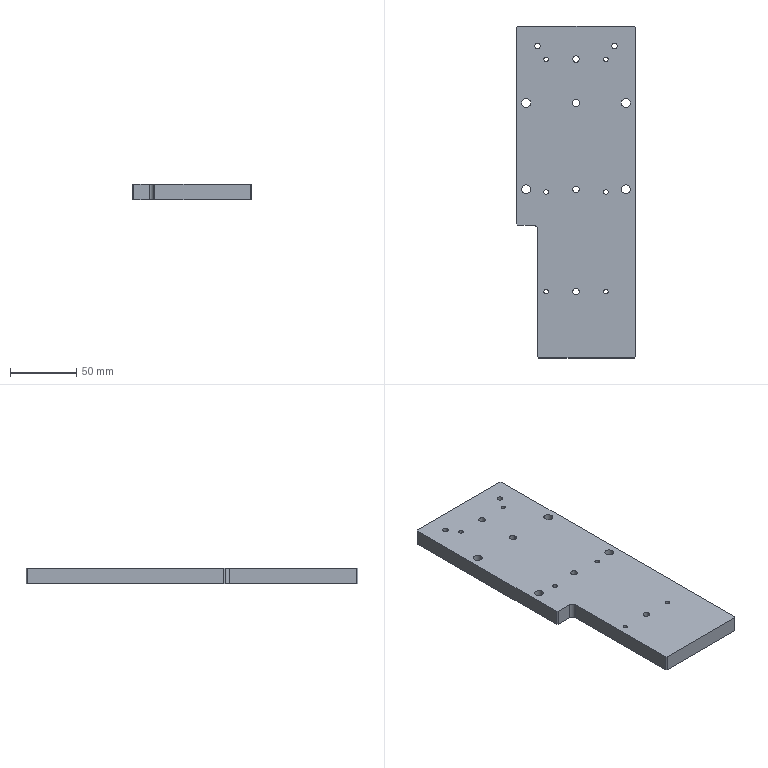Part | NX | 1 solid | 41 faces | box 90 x 250 x 12 mm | volume 245643 mm3 | cylinder 22 | plane 19 | commonest cylinder face diameters 3.3 x6 5 x5 6.6 x4 11 x4 4.2 x2 6 x1
STEP:
#1=CARTESIAN_POINT('',(-29.,97.,0.));
#2=VERTEX_POINT('',#1);
#3=CARTESIAN_POINT('',(-32.,100.,0.));
#4=VERTEX_POINT('',#3);
#5=CARTESIAN_POINT('',(-32.,97.,0.));
#6=DIRECTION('',(0.,0.,1.));
#7=DIRECTION('',(-1.,0.,0.));
#8=AXIS2_PLACEMENT_3D('',#5,#6,#7);
#9=CIRCLE('',#8,3.);
#10=EDGE_CURVE('',#2,#4,#9,.T.);
#11=ORIENTED_EDGE('',*,*,#10,.F.);
#12=CARTESIAN_POINT('',(-29.,97.,12.));
#13=VERTEX_POINT('',#12);
#14=CARTESIAN_POINT('',(-29.,97.,0.));
#15=DIRECTION('',(0.,0.,-1.));
#16=VECTOR('',#15,1000.);
#17=LINE('',#14,#16);
#18=EDGE_CURVE('',#13,#2,#17,.T.);
#19=ORIENTED_EDGE('',*,*,#18,.F.);
#20=CARTESIAN_POINT('',(-32.,100.,12.));
#21=VERTEX_POINT('',#20);
#22=CARTESIAN_POINT('',(-32.,97.,12.));
#23=DIRECTION('',(0.,0.,-1.));
#24=DIRECTION('',(-1.,0.,0.));
#25=AXIS2_PLACEMENT_3D('',#22,#23,#24);
#26=CIRCLE('',#25,3.);
#27=EDGE_CURVE('',#21,#13,#26,.T.);
#28=ORIENTED_EDGE('',*,*,#27,.F.);
#29=CARTESIAN_POINT('',(-32.,100.,12.));
#30=DIRECTION('',(0.,0.,1.));
#31=VECTOR('',#30,1000.);
#32=LINE('',#29,#31);
#33=EDGE_CURVE('',#4,#21,#32,.T.);
#34=ORIENTED_EDGE('',*,*,#33,.F.);
#35=EDGE_LOOP('',(#11,#19,#28,#34));
#36=FACE_BOUND('',#35,.T.);
#37=CARTESIAN_POINT('',(-32.,97.,0.));
#38=DIRECTION('',(0.,0.,-1.));
#39=DIRECTION('',(-1.,0.,0.));
#40=AXIS2_PLACEMENT_3D('',#37,#38,#39);
#41=CYLINDRICAL_SURFACE('',#40,3.);
#42=ADVANCED_FACE('',(#36),#41,.F.);
#43=CARTESIAN_POINT('',(45.,249.,12.));
#44=VERTEX_POINT('',#43);
#45=CARTESIAN_POINT('',(44.,250.,12.));
#46=VERTEX_POINT('',#45);
#47=CARTESIAN_POINT('',(44.,250.,12.));
#48=DIRECTION('',(-0.7071,0.7071,0.));
#49=VECTOR('',#48,1000.);
#50=LINE('',#47,#49);
#51=EDGE_CURVE('',#44,#46,#50,.T.);
#52=ORIENTED_EDGE('',*,*,#51,.F.);
#53=CARTESIAN_POINT('',(45.,249.,0.));
#54=VERTEX_POINT('',#53);
#55=CARTESIAN_POINT('',(45.,249.,12.));
#56=DIRECTION('',(0.,0.,1.));
#57=VECTOR('',#56,1000.);
#58=LINE('',#55,#57);
#59=EDGE_CURVE('',#54,#44,#58,.T.);
#60=ORIENTED_EDGE('',*,*,#59,.F.);
#61=CARTESIAN_POINT('',(44.,250.,0.));
#62=VERTEX_POINT('',#61);
#63=CARTESIAN_POINT('',(147.,147.,0.));
#64=DIRECTION('',(0.7071,-0.7071,0.));
#65=VECTOR('',#64,1000.);
#66=LINE('',#63,#65);
#67=EDGE_CURVE('',#62,#54,#66,.T.);
#68=ORIENTED_EDGE('',*,*,#67,.F.);
#69=CARTESIAN_POINT('',(44.,250.,12.));
#70=DIRECTION('',(0.,0.,-1.));
#71=VECTOR('',#70,1000.);
#72=LINE('',#69,#71);
#73=EDGE_CURVE('',#46,#62,#72,.T.);
#74=ORIENTED_EDGE('',*,*,#73,.F.);
#75=EDGE_LOOP('',(#52,#60,#68,#74));
#76=FACE_BOUND('',#75,.T.);
#77=CARTESIAN_POINT('',(44.,250.,12.));
#78=DIRECTION('',(-0.7071,-0.7071,0.));
#79=DIRECTION('',(0.,0.,-1.));
#80=AXIS2_PLACEMENT_3D('',#77,#78,#79);
#81=PLANE('',#80);
#82=ADVANCED_FACE('',(#76),#81,.F.);
#83=CARTESIAN_POINT('',(-44.,250.,12.));
#84=VERTEX_POINT('',#83);
#85=CARTESIAN_POINT('',(-45.,249.,12.));
#86=VERTEX_POINT('',#85);
#87=CARTESIAN_POINT('',(-45.,249.,12.));
#88=DIRECTION('',(-0.7071,-0.7071,0.));
#89=VECTOR('',#88,1000.);
#90=LINE('',#87,#89);
#91=EDGE_CURVE('',#84,#86,#90,.T.);
#92=ORIENTED_EDGE('',*,*,#91,.F.);
#93=CARTESIAN_POINT('',(-44.,250.,0.));
#94=VERTEX_POINT('',#93);
#95=CARTESIAN_POINT('',(-44.,250.,12.));
#96=DIRECTION('',(0.,0.,1.));
#97=VECTOR('',#96,1000.);
#98=LINE('',#95,#97);
#99=EDGE_CURVE('',#94,#84,#98,.T.);
#100=ORIENTED_EDGE('',*,*,#99,.F.);
#101=CARTESIAN_POINT('',(-45.,249.,0.));
#102=VERTEX_POINT('',#101);
#103=CARTESIAN_POINT('',(-147.,147.,0.));
#104=DIRECTION('',(0.7071,0.7071,0.));
#105=VECTOR('',#104,1000.);
#106=LINE('',#103,#105);
#107=EDGE_CURVE('',#102,#94,#106,.T.);
#108=ORIENTED_EDGE('',*,*,#107,.F.);
#109=CARTESIAN_POINT('',(-45.,249.,12.));
#110=DIRECTION('',(0.,0.,-1.));
#111=VECTOR('',#110,1000.);
#112=LINE('',#109,#111);
#113=EDGE_CURVE('',#86,#102,#112,.T.);
#114=ORIENTED_EDGE('',*,*,#113,.F.);
#115=EDGE_LOOP('',(#92,#100,#108,#114));
#116=FACE_BOUND('',#115,.T.);
#117=CARTESIAN_POINT('',(-45.,249.,12.));
#118=DIRECTION('',(0.7071,-0.7071,0.));
#119=DIRECTION('',(0.,0.,-1.));
#120=AXIS2_PLACEMENT_3D('',#117,#118,#119);
#121=PLANE('',#120);
#122=ADVANCED_FACE('',(#116),#121,.F.);
#123=CARTESIAN_POINT('',(44.,0.,12.));
#124=VERTEX_POINT('',#123);
#125=CARTESIAN_POINT('',(45.,1.,12.));
#126=VERTEX_POINT('',#125);
#127=CARTESIAN_POINT('',(45.,1.,12.));
#128=DIRECTION('',(0.7071,0.7071,0.));
#129=VECTOR('',#128,1000.);
#130=LINE('',#127,#129);
#131=EDGE_CURVE('',#124,#126,#130,.T.);
#132=ORIENTED_EDGE('',*,*,#131,.F.);
#133=CARTESIAN_POINT('',(44.,0.,0.));
#134=VERTEX_POINT('',#133);
#135=CARTESIAN_POINT('',(44.,0.,12.));
#136=DIRECTION('',(0.,0.,1.));
#137=VECTOR('',#136,1000.);
#138=LINE('',#135,#137);
#139=EDGE_CURVE('',#134,#124,#138,.T.);
#140=ORIENTED_EDGE('',*,*,#139,.F.);
#141=CARTESIAN_POINT('',(45.,1.,0.));
#142=VERTEX_POINT('',#141);
#143=CARTESIAN_POINT('',(22.,-22.,0.));
#144=DIRECTION('',(-0.7071,-0.7071,0.));
#145=VECTOR('',#144,1000.);
#146=LINE('',#143,#145);
#147=EDGE_CURVE('',#142,#134,#146,.T.);
#148=ORIENTED_EDGE('',*,*,#147,.F.);
#149=CARTESIAN_POINT('',(45.,1.,12.));
#150=DIRECTION('',(0.,0.,-1.));
#151=VECTOR('',#150,1000.);
#152=LINE('',#149,#151);
#153=EDGE_CURVE('',#126,#142,#152,.T.);
#154=ORIENTED_EDGE('',*,*,#153,.F.);
#155=EDGE_LOOP('',(#132,#140,#148,#154));
#156=FACE_BOUND('',#155,.T.);
#157=CARTESIAN_POINT('',(45.,1.,12.));
#158=DIRECTION('',(-0.7071,0.7071,0.));
#159=DIRECTION('',(0.,0.,-1.));
#160=AXIS2_PLACEMENT_3D('',#157,#158,#159);
#161=PLANE('',#160);
#162=ADVANCED_FACE('',(#156),#161,.F.);
#163=CARTESIAN_POINT('',(-44.,100.,0.));
#164=VERTEX_POINT('',#163);
#165=CARTESIAN_POINT('',(-45.,101.,0.));
#166=VERTEX_POINT('',#165);
#167=CARTESIAN_POINT('',(28.,28.,0.));
#168=DIRECTION('',(-0.7071,0.7071,0.));
#169=VECTOR('',#168,1000.);
#170=LINE('',#167,#169);
#171=EDGE_CURVE('',#164,#166,#170,.T.);
#172=ORIENTED_EDGE('',*,*,#171,.F.);
#173=CARTESIAN_POINT('',(-44.,100.,12.));
#174=VERTEX_POINT('',#173);
#175=CARTESIAN_POINT('',(-44.,100.,0.));
#176=DIRECTION('',(0.,0.,-1.));
#177=VECTOR('',#176,1000.);
#178=LINE('',#175,#177);
#179=EDGE_CURVE('',#174,#164,#178,.T.);
#180=ORIENTED_EDGE('',*,*,#179,.F.);
#181=CARTESIAN_POINT('',(-45.,101.,12.));
#182=VERTEX_POINT('',#181);
#183=CARTESIAN_POINT('',(-45.,101.,12.));
#184=DIRECTION('',(0.7071,-0.7071,0.));
#185=VECTOR('',#184,1000.);
#186=LINE('',#183,#185);
#187=EDGE_CURVE('',#182,#174,#186,.T.);
#188=ORIENTED_EDGE('',*,*,#187,.F.);
#189=CARTESIAN_POINT('',(-45.,101.,12.));
#190=DIRECTION('',(0.,0.,1.));
#191=VECTOR('',#190,1000.);
#192=LINE('',#189,#191);
#193=EDGE_CURVE('',#166,#182,#192,.T.);
#194=ORIENTED_EDGE('',*,*,#193,.F.);
#195=EDGE_LOOP('',(#172,#180,#188,#194));
#196=FACE_BOUND('',#195,.T.);
#197=CARTESIAN_POINT('',(-45.,101.,12.));
#198=DIRECTION('',(0.7071,0.7071,0.));
#199=DIRECTION('',(0.,0.,1.));
#200=AXIS2_PLACEMENT_3D('',#197,#198,#199);
#201=PLANE('',#200);
#202=ADVANCED_FACE('',(#196),#201,.F.);
#203=CARTESIAN_POINT('',(-28.,0.,0.));
#204=VERTEX_POINT('',#203);
#205=CARTESIAN_POINT('',(-29.,1.,0.));
#206=VERTEX_POINT('',#205);
#207=CARTESIAN_POINT('',(-14.,-14.,0.));
#208=DIRECTION('',(-0.7071,0.7071,0.));
#209=VECTOR('',#208,1000.);
#210=LINE('',#207,#209);
#211=EDGE_CURVE('',#204,#206,#210,.T.);
#212=ORIENTED_EDGE('',*,*,#211,.F.);
#213=CARTESIAN_POINT('',(-28.,0.,12.));
#214=VERTEX_POINT('',#213);
#215=CARTESIAN_POINT('',(-28.,0.,12.));
#216=DIRECTION('',(0.,0.,-1.));
#217=VECTOR('',#216,1000.);
#218=LINE('',#215,#217);
#219=EDGE_CURVE('',#214,#204,#218,.T.);
#220=ORIENTED_EDGE('',*,*,#219,.F.);
#221=CARTESIAN_POINT('',(-29.,1.,12.));
#222=VERTEX_POINT('',#221);
#223=CARTESIAN_POINT('',(-29.,1.,12.));
#224=DIRECTION('',(0.7071,-0.7071,0.));
#225=VECTOR('',#224,1000.);
#226=LINE('',#223,#225);
#227=EDGE_CURVE('',#222,#214,#226,.T.);
#228=ORIENTED_EDGE('',*,*,#227,.F.);
#229=CARTESIAN_POINT('',(-29.,1.,0.));
#230=DIRECTION('',(0.,0.,1.));
#231=VECTOR('',#230,1000.);
#232=LINE('',#229,#231);
#233=EDGE_CURVE('',#206,#222,#232,.T.);
#234=ORIENTED_EDGE('',*,*,#233,.F.);
#235=EDGE_LOOP('',(#212,#220,#228,#234));
#236=FACE_BOUND('',#235,.T.);
#237=CARTESIAN_POINT('',(-29.,1.,0.));
#238=DIRECTION('',(0.7071,0.7071,0.));
#239=DIRECTION('',(0.,0.,1.));
#240=AXIS2_PLACEMENT_3D('',#237,#238,#239);
#241=PLANE('',#240);
#242=ADVANCED_FACE('',(#236),#241,.F.);
#243=CARTESIAN_POINT('',(-29.,100.,12.));
#244=DIRECTION('',(0.,1.,0.));
#245=VECTOR('',#244,1000.);
#246=LINE('',#243,#245);
#247=EDGE_CURVE('',#222,#13,#246,.T.);
#248=ORIENTED_EDGE('',*,*,#247,.T.);
#249=ORIENTED_EDGE('',*,*,#18,.T.);
#250=CARTESIAN_POINT('',(-29.,100.,0.));
#251=DIRECTION('',(0.,1.,0.));
#252=VECTOR('',#251,1000.);
#253=LINE('',#250,#252);
#254=EDGE_CURVE('',#206,#2,#253,.T.);
#255=ORIENTED_EDGE('',*,*,#254,.F.);
#256=ORIENTED_EDGE('',*,*,#233,.T.);
#257=EDGE_LOOP('',(#248,#249,#255,#256));
#258=FACE_BOUND('',#257,.T.);
#259=CARTESIAN_POINT('',(-29.,100.,0.));
#260=DIRECTION('',(1.,0.,0.));
#261=DIRECTION('',(0.,1.,0.));
#262=AXIS2_PLACEMENT_3D('',#259,#260,#261);
#263=PLANE('',#262);
#264=ADVANCED_FACE('',(#258),#263,.F.);
#265=CARTESIAN_POINT('',(-45.,100.,0.));
#266=DIRECTION('',(-1.,0.,0.));
#267=VECTOR('',#266,1000.);
#268=LINE('',#265,#267);
#269=EDGE_CURVE('',#4,#164,#268,.T.);
#270=ORIENTED_EDGE('',*,*,#269,.F.);
#271=ORIENTED_EDGE('',*,*,#33,.T.);
#272=CARTESIAN_POINT('',(-45.,100.,12.));
#273=DIRECTION('',(-1.,0.,0.));
#274=VECTOR('',#273,1000.);
#275=LINE('',#272,#274);
#276=EDGE_CURVE('',#21,#174,#275,.T.);
#277=ORIENTED_EDGE('',*,*,#276,.T.);
#278=ORIENTED_EDGE('',*,*,#179,.T.);
#279=EDGE_LOOP('',(#270,#271,#277,#278));
#280=FACE_BOUND('',#279,.T.);
#281=CARTESIAN_POINT('',(-45.,100.,0.));
#282=DIRECTION('',(0.,1.,0.));
#283=DIRECTION('',(0.,0.,1.));
#284=AXIS2_PLACEMENT_3D('',#281,#282,#283);
#285=PLANE('',#284);
#286=ADVANCED_FACE('',(#280),#285,.F.);
#287=CARTESIAN_POINT('',(-2.5,192.5,0.));
#288=VERTEX_POINT('',#287);
#289=CARTESIAN_POINT('',(-2.5,192.5,12.));
#290=VERTEX_POINT('',#289);
#291=CARTESIAN_POINT('',(-2.5,192.5,0.));
#292=DIRECTION('',(0.,0.,1.));
#293=VECTOR('',#292,1000.);
#294=LINE('',#291,#293);
#295=EDGE_CURVE('',#288,#290,#294,.T.);
#296=ORIENTED_EDGE('',*,*,#295,.T.);
#297=CARTESIAN_POINT('',(-2.5,191.5,12.));
#298=VERTEX_POINT('',#297);
#299=CARTESIAN_POINT('',(-2.5,191.5,12.));
#300=DIRECTION('',(0.,1.,0.));
#301=VECTOR('',#300,1000.);
#302=LINE('',#299,#301);
#303=EDGE_CURVE('',#298,#290,#302,.T.);
#304=ORIENTED_EDGE('',*,*,#303,.F.);
#305=CARTESIAN_POINT('',(-2.5,191.5,0.));
#306=VERTEX_POINT('',#305);
#307=CARTESIAN_POINT('',(-2.5,191.5,0.));
#308=DIRECTION('',(0.,0.,-1.));
#309=VECTOR('',#308,1000.);
#310=LINE('',#307,#309);
#311=EDGE_CURVE('',#298,#306,#310,.T.);
#312=ORIENTED_EDGE('',*,*,#311,.T.);
#313=CARTESIAN_POINT('',(-2.5,191.5,0.));
#314=DIRECTION('',(0.,1.,0.));
#315=VECTOR('',#314,1000.);
#316=LINE('',#313,#315);
#317=EDGE_CURVE('',#306,#288,#316,.T.);
#318=ORIENTED_EDGE('',*,*,#317,.T.);
#319=EDGE_LOOP('',(#296,#304,#312,#318));
#320=FACE_BOUND('',#319,.T.);
#321=CARTESIAN_POINT('',(-2.5,191.5,0.));
#322=DIRECTION('',(-1.,0.,0.));
#323=DIRECTION('',(0.,0.,1.));
#324=AXIS2_PLACEMENT_3D('',#321,#322,#323);
#325=PLANE('',#324);
#326=ADVANCED_FACE('',(#320),#325,.F.);
#327=CARTESIAN_POINT('',(2.5,192.5,0.));
#328=VERTEX_POINT('',#327);
#329=CARTESIAN_POINT('',(2.5,192.5,12.));
#330=VERTEX_POINT('',#329);
#331=CARTESIAN_POINT('',(2.5,192.5,12.));
#332=DIRECTION('',(0.,0.,1.));
#333=VECTOR('',#332,1000.);
#334=LINE('',#331,#333);
#335=EDGE_CURVE('',#328,#330,#334,.T.);
#336=ORIENTED_EDGE('',*,*,#335,.F.);
#337=CARTESIAN_POINT('',(2.5,191.5,0.));
#338=VERTEX_POINT('',#337);
#339=CARTESIAN_POINT('',(2.5,191.5,0.));
#340=DIRECTION('',(0.,1.,0.));
#341=VECTOR('',#340,1000.);
#342=LINE('',#339,#341);
#343=EDGE_CURVE('',#338,#328,#342,.T.);
#344=ORIENTED_EDGE('',*,*,#343,.F.);
#345=CARTESIAN_POINT('',(2.5,191.5,12.));
#346=VERTEX_POINT('',#345);
#347=CARTESIAN_POINT('',(2.5,191.5,12.));
#348=DIRECTION('',(0.,0.,1.));
#349=VECTOR('',#348,1000.);
#350=LINE('',#347,#349);
#351=EDGE_CURVE('',#338,#346,#350,.T.);
#352=ORIENTED_EDGE('',*,*,#351,.T.);
#353=CARTESIAN_POINT('',(2.5,191.5,12.));
#354=DIRECTION('',(0.,1.,0.));
#355=VECTOR('',#354,1000.);
#356=LINE('',#353,#355);
#357=EDGE_CURVE('',#346,#330,#356,.T.);
#358=ORIENTED_EDGE('',*,*,#357,.T.);
#359=EDGE_LOOP('',(#336,#344,#352,#358));
#360=FACE_BOUND('',#359,.T.);
#361=CARTESIAN_POINT('',(2.5,191.5,12.));
#362=DIRECTION('',(-1.,0.,0.));
#363=DIRECTION('',(0.,0.,1.));
#364=AXIS2_PLACEMENT_3D('',#361,#362,#363);
#365=PLANE('',#364);
#366=ADVANCED_FACE('',(#360),#365,.T.);
#367=CARTESIAN_POINT('',(0.,191.5,12.));
#368=DIRECTION('',(0.,0.,-1.));
#369=DIRECTION('',(-1.,0.,0.));
#370=AXIS2_PLACEMENT_3D('',#367,#368,#369);
#371=CIRCLE('',#370,2.5);
#372=EDGE_CURVE('',#346,#298,#371,.T.);
#373=ORIENTED_EDGE('',*,*,#372,.F.);
#374=ORIENTED_EDGE('',*,*,#351,.F.);
#375=CARTESIAN_POINT('',(0.,191.5,0.));
#376=DIRECTION('',(0.,0.,-1.));
#377=DIRECTION('',(-1.,0.,0.));
#378=AXIS2_PLACEMENT_3D('',#375,#376,#377);
#379=CIRCLE('',#378,2.5);
#380=EDGE_CURVE('',#338,#306,#379,.T.);
#381=ORIENTED_EDGE('',*,*,#380,.T.);
#382=ORIENTED_EDGE('',*,*,#311,.F.);
#383=EDGE_LOOP('',(#373,#374,#381,#382));
#384=FACE_BOUND('',#383,.T.);
#385=CARTESIAN_POINT('',(0.,191.5,0.));
#386=DIRECTION('',(0.,0.,-1.));
#387=DIRECTION('',(-1.,0.,0.));
#388=AXIS2_PLACEMENT_3D('',#385,#386,#387);
#389=CYLINDRICAL_SURFACE('',#388,2.5);
#390=ADVANCED_FACE('',(#384),#389,.F.);
#391=CARTESIAN_POINT('',(0.,192.5,0.));
#392=DIRECTION('',(0.,0.,-1.));
#393=DIRECTION('',(-1.,0.,0.));
#394=AXIS2_PLACEMENT_3D('',#391,#392,#393);
#395=CIRCLE('',#394,2.5);
#396=EDGE_CURVE('',#288,#328,#395,.T.);
#397=ORIENTED_EDGE('',*,*,#396,.T.);
#398=ORIENTED_EDGE('',*,*,#335,.T.);
#399=CARTESIAN_POINT('',(0.,192.5,12.));
#400=DIRECTION('',(0.,0.,-1.));
#401=DIRECTION('',(-1.,0.,0.));
#402=AXIS2_PLACEMENT_3D('',#399,#400,#401);
#403=CIRCLE('',#402,2.5);
#404=EDGE_CURVE('',#290,#330,#403,.T.);
#405=ORIENTED_EDGE('',*,*,#404,.F.);
#406=ORIENTED_EDGE('',*,*,#295,.F.);
#407=EDGE_LOOP('',(#397,#398,#405,#406));
#408=FACE_BOUND('',#407,.T.);
#409=CARTESIAN_POINT('',(0.,192.5,0.));
#410=DIRECTION('',(0.,0.,-1.));
#411=DIRECTION('',(-1.,0.,0.));
#412=AXIS2_PLACEMENT_3D('',#409,#410,#411);
#413=CYLINDRICAL_SURFACE('',#412,2.5);
#414=ADVANCED_FACE('',(#408),#413,.F.);
#415=CARTESIAN_POINT('',(32.,127.,6.4));
#416=VERTEX_POINT('',#415);
#417=CARTESIAN_POINT('',(37.5,127.,6.4));
#418=DIRECTION('',(0.,0.,-1.));
#419=DIRECTION('',(-1.,0.,0.));
#420=AXIS2_PLACEMENT_3D('',#417,#418,#419);
#421=CIRCLE('',#420,5.5);
#422=EDGE_CURVE('',#416,#416,#421,.T.);
#423=ORIENTED_EDGE('',*,*,#422,.T.);
#424=EDGE_LOOP('',(#423));
#425=FACE_BOUND('',#424,.T.);
#426=CARTESIAN_POINT('',(34.2,127.,6.4));
#427=VERTEX_POINT('',#426);
#428=CARTESIAN_POINT('',(37.5,127.,6.4));
#429=DIRECTION('',(0.,0.,-1.));
#430=DIRECTION('',(-1.,0.,0.));
#431=AXIS2_PLACEMENT_3D('',#428,#429,#430);
#432=CIRCLE('',#431,3.3);
#433=EDGE_CURVE('',#427,#427,#432,.T.);
#434=ORIENTED_EDGE('',*,*,#433,.F.);
#435=EDGE_LOOP('',(#434));
#436=FACE_BOUND('',#435,.T.);
#437=CARTESIAN_POINT('',(40.8,127.,6.4));
#438=DIRECTION('',(0.,0.,1.));
#439=DIRECTION('',(1.,0.,0.));
#440=AXIS2_PLACEMENT_3D('',#437,#438,#439);
#441=PLANE('',#440);
#442=ADVANCED_FACE('',(#425,#436),#441,.F.);
#443=CARTESIAN_POINT('',(-32.,192.,6.4));
#444=VERTEX_POINT('',#443);
#445=CARTESIAN_POINT('',(-37.5,192.,6.4));
#446=DIRECTION('',(0.,0.,-1.));
#447=DIRECTION('',(1.,0.,0.));
#448=AXIS2_PLACEMENT_3D('',#445,#446,#447);
#449=CIRCLE('',#448,5.5);
#450=EDGE_CURVE('',#444,#444,#449,.T.);
#451=ORIENTED_EDGE('',*,*,#450,.T.);
#452=EDGE_LOOP('',(#451));
#453=FACE_BOUND('',#452,.T.);
#454=CARTESIAN_POINT('',(-34.2,192.,6.4));
#455=VERTEX_POINT('',#454);
#456=CARTESIAN_POINT('',(-37.5,192.,6.4));
#457=DIRECTION('',(0.,0.,-1.));
#458=DIRECTION('',(1.,0.,0.));
#459=AXIS2_PLACEMENT_3D('',#456,#457,#458);
#460=CIRCLE('',#459,3.3);
#461=EDGE_CURVE('',#455,#455,#460,.T.);
#462=ORIENTED_EDGE('',*,*,#461,.F.);
#463=EDGE_LOOP('',(#462));
#464=FACE_BOUND('',#463,.T.);
#465=CARTESIAN_POINT('',(40.8,127.,6.4));
#466=DIRECTION('',(0.,0.,1.));
#467=DIRECTION('',(1.,0.,0.));
#468=AXIS2_PLACEMENT_3D('',#465,#466,#467);
#469=PLANE('',#468);
#470=ADVANCED_FACE('',(#453,#464),#469,.F.);
#471=CARTESIAN_POINT('',(43.,192.,6.4));
#472=VERTEX_POINT('',#471);
#473=CARTESIAN_POINT('',(37.5,192.,6.4));
#474=DIRECTION('',(0.,0.,-1.));
#475=DIRECTION('',(1.,0.,0.));
#476=AXIS2_PLACEMENT_3D('',#473,#474,#475);
#477=CIRCLE('',#476,5.5);
#478=EDGE_CURVE('',#472,#472,#477,.T.);
#479=ORIENTED_EDGE('',*,*,#478,.T.);
#480=EDGE_LOOP('',(#479));
#481=FACE_BOUND('',#480,.T.);
#482=CARTESIAN_POINT('',(40.8,192.,6.4));
#483=VERTEX_POINT('',#482);
#484=CARTESIAN_POINT('',(37.5,192.,6.4));
#485=DIRECTION('',(0.,0.,-1.));
#486=DIRECTION('',(1.,0.,0.));
#487=AXIS2_PLACEMENT_3D('',#484,#485,#486);
#488=CIRCLE('',#487,3.3);
#489=EDGE_CURVE('',#483,#483,#488,.T.);
#490=ORIENTED_EDGE('',*,*,#489,.F.);
#491=EDGE_LOOP('',(#490));
#492=FACE_BOUND('',#491,.T.);
#493=CARTESIAN_POINT('',(40.8,127.,6.4));
#494=DIRECTION('',(0.,0.,1.));
#495=DIRECTION('',(1.,0.,0.));
#496=AXIS2_PLACEMENT_3D('',#493,#494,#495);
#497=PLANE('',#496);
#498=ADVANCED_FACE('',(#481,#492),#497,.F.);
#499=CARTESIAN_POINT('',(-32.,127.,6.4));
#500=VERTEX_POINT('',#499);
#501=CARTESIAN_POINT('',(-37.5,127.,6.4));
#502=DIRECTION('',(0.,0.,-1.));
#503=DIRECTION('',(1.,0.,0.));
#504=AXIS2_PLACEMENT_3D('',#501,#502,#503);
#505=CIRCLE('',#504,5.5);
#506=EDGE_CURVE('',#500,#500,#505,.T.);
#507=ORIENTED_EDGE('',*,*,#506,.T.);
#508=EDGE_LOOP('',(#507));
#509=FACE_BOUND('',#508,.T.);
#510=CARTESIAN_POINT('',(-34.2,127.,6.4));
#511=VERTEX_POINT('',#510);
#512=CARTESIAN_POINT('',(-37.5,127.,6.4));
#513=DIRECTION('',(0.,0.,-1.));
#514=DIRECTION('',(1.,0.,0.));
#515=AXIS2_PLACEMENT_3D('',#512,#513,#514);
#516=CIRCLE('',#515,3.3);
#517=EDGE_CURVE('',#511,#511,#516,.T.);
#518=ORIENTED_EDGE('',*,*,#517,.F.);
#519=EDGE_LOOP('',(#518));
#520=FACE_BOUND('',#519,.T.);
#521=CARTESIAN_POINT('',(40.8,127.,6.4));
#522=DIRECTION('',(0.,0.,1.));
#523=DIRECTION('',(1.,0.,0.));
#524=AXIS2_PLACEMENT_3D('',#521,#522,#523);
#525=PLANE('',#524);
#526=ADVANCED_FACE('',(#509,#520),#525,.F.);
#527=ORIENTED_EDGE('',*,*,#247,.F.);
#528=ORIENTED_EDGE('',*,*,#227,.T.);
#529=CARTESIAN_POINT('',(-45.,0.,12.));
#530=DIRECTION('',(1.,0.,0.));
#531=VECTOR('',#530,1000.);
#532=LINE('',#529,#531);
#533=EDGE_CURVE('',#214,#124,#532,.T.);
#534=ORIENTED_EDGE('',*,*,#533,.T.);
#535=ORIENTED_EDGE('',*,*,#131,.T.);
#536=CARTESIAN_POINT('',(45.,0.,12.));
#537=DIRECTION('',(0.,1.,0.));
#538=VECTOR('',#537,1000.);
#539=LINE('',#536,#538);
#540=EDGE_CURVE('',#126,#44,#539,.T.);
#541=ORIENTED_EDGE('',*,*,#540,.T.);
#542=ORIENTED_EDGE('',*,*,#51,.T.);
#543=CARTESIAN_POINT('',(-45.,250.,12.));
#544=DIRECTION('',(-1.,0.,0.));
#545=VECTOR('',#544,1000.);
#546=LINE('',#543,#545);
#547=EDGE_CURVE('',#46,#84,#546,.T.);
#548=ORIENTED_EDGE('',*,*,#547,.T.);
#549=ORIENTED_EDGE('',*,*,#91,.T.);
#550=CARTESIAN_POINT('',(-45.,0.,12.));
#551=DIRECTION('',(0.,-1.,0.));
#552=VECTOR('',#551,1000.);
#553=LINE('',#550,#552);
#554=EDGE_CURVE('',#86,#182,#553,.T.);
#555=ORIENTED_EDGE('',*,*,#554,.T.);
#556=ORIENTED_EDGE('',*,*,#187,.T.);
#557=ORIENTED_EDGE('',*,*,#276,.F.);
#558=ORIENTED_EDGE('',*,*,#27,.T.);
#559=EDGE_LOOP('',(#527,#528,#534,#535,#541,#542,#548,#549,#555,#556,#557,#558));
#560=FACE_BOUND('',#559,.T.);
#561=CARTESIAN_POINT('',(-24.15,125.,12.));
#562=VERTEX_POINT('',#561);
#563=CARTESIAN_POINT('',(-22.5,125.,12.));
#564=DIRECTION('',(0.,0.,-1.));
#565=DIRECTION('',(-1.,0.,0.));
#566=AXIS2_PLACEMENT_3D('',#563,#564,#565);
#567=CIRCLE('',#566,1.65);
#568=EDGE_CURVE('',#562,#562,#567,.T.);
#569=ORIENTED_EDGE('',*,*,#568,.T.);
#570=EDGE_LOOP('',(#569));
#571=FACE_BOUND('',#570,.T.);
#572=CARTESIAN_POINT('',(-24.15,50.,12.));
#573=VERTEX_POINT('',#572);
#574=CARTESIAN_POINT('',(-22.5,50.,12.));
#575=DIRECTION('',(0.,0.,-1.));
#576=DIRECTION('',(-1.,0.,0.));
#577=AXIS2_PLACEMENT_3D('',#574,#575,#576);
#578=CIRCLE('',#577,1.65);
#579=EDGE_CURVE('',#573,#573,#578,.T.);
#580=ORIENTED_EDGE('',*,*,#579,.T.);
#581=EDGE_LOOP('',(#580));
#582=FACE_BOUND('',#581,.T.);
#583=CARTESIAN_POINT('',(20.85,125.,12.));
#584=VERTEX_POINT('',#583);
#585=CARTESIAN_POINT('',(22.5,125.,12.));
#586=DIRECTION('',(0.,0.,-1.));
#587=DIRECTION('',(-1.,0.,0.));
#588=AXIS2_PLACEMENT_3D('',#585,#586,#587);
#589=CIRCLE('',#588,1.65);
#590=EDGE_CURVE('',#584,#584,#589,.T.);
#591=ORIENTED_EDGE('',*,*,#590,.T.);
#592=EDGE_LOOP('',(#591));
#593=FACE_BOUND('',#592,.T.);
#594=CARTESIAN_POINT('',(20.85,50.,12.));
#595=VERTEX_POINT('',#594);
#596=CARTESIAN_POINT('',(22.5,50.,12.));
#597=DIRECTION('',(0.,0.,-1.));
#598=DIRECTION('',(-1.,0.,0.));
#599=AXIS2_PLACEMENT_3D('',#596,#597,#598);
#600=CIRCLE('',#599,1.65);
#601=EDGE_CURVE('',#595,#595,#600,.T.);
#602=ORIENTED_EDGE('',*,*,#601,.T.);
#603=EDGE_LOOP('',(#602));
#604=FACE_BOUND('',#603,.T.);
#605=CARTESIAN_POINT('',(20.85,225.,12.));
#606=VERTEX_POINT('',#605);
#607=CARTESIAN_POINT('',(22.5,225.,12.));
#608=DIRECTION('',(0.,0.,-1.));
#609=DIRECTION('',(-1.,0.,0.));
#610=AXIS2_PLACEMENT_3D('',#607,#608,#609);
#611=CIRCLE('',#610,1.65);
#612=EDGE_CURVE('',#606,#606,#611,.T.);
#613=ORIENTED_EDGE('',*,*,#612,.T.);
#614=EDGE_LOOP('',(#613));
#615=FACE_BOUND('',#614,.T.);
#616=CARTESIAN_POINT('',(-24.15,225.,12.));
#617=VERTEX_POINT('',#616);
#618=CARTESIAN_POINT('',(-22.5,225.,12.));
#619=DIRECTION('',(0.,0.,-1.));
#620=DIRECTION('',(-1.,0.,0.));
#621=AXIS2_PLACEMENT_3D('',#618,#619,#620);
#622=CIRCLE('',#621,1.65);
#623=EDGE_CURVE('',#617,#617,#622,.T.);
#624=ORIENTED_EDGE('',*,*,#623,.T.);
#625=EDGE_LOOP('',(#624));
#626=FACE_BOUND('',#625,.T.);
#627=CARTESIAN_POINT('',(31.1,235.,12.));
#628=VERTEX_POINT('',#627);
#629=CARTESIAN_POINT('',(29.,235.,12.));
#630=DIRECTION('',(0.,0.,1.));
#631=DIRECTION('',(1.,0.,0.));
#632=AXIS2_PLACEMENT_3D('',#629,#630,#631);
#633=CIRCLE('',#632,2.1);
#634=EDGE_CURVE('',#628,#628,#633,.T.);
#635=ORIENTED_EDGE('',*,*,#634,.F.);
#636=EDGE_LOOP('',(#635));
#637=FACE_BOUND('',#636,.T.);
#638=CARTESIAN_POINT('',(-26.9,235.,12.));
#639=VERTEX_POINT('',#638);
#640=CARTESIAN_POINT('',(-29.,235.,12.));
#641=DIRECTION('',(0.,0.,1.));
#642=DIRECTION('',(1.,0.,0.));
#643=AXIS2_PLACEMENT_3D('',#640,#641,#642);
#644=CIRCLE('',#643,2.1);
#645=EDGE_CURVE('',#639,#639,#644,.T.);
#646=ORIENTED_EDGE('',*,*,#645,.F.);
#647=EDGE_LOOP('',(#646));
#648=FACE_BOUND('',#647,.T.);
#649=CARTESIAN_POINT('',(-40.8,127.,12.));
#650=VERTEX_POINT('',#649);
#651=CARTESIAN_POINT('',(-37.5,127.,12.));
#652=DIRECTION('',(0.,0.,-1.));
#653=DIRECTION('',(-1.,0.,0.));
#654=AXIS2_PLACEMENT_3D('',#651,#652,#653);
#655=CIRCLE('',#654,3.3);
#656=EDGE_CURVE('',#650,#650,#655,.T.);
#657=ORIENTED_EDGE('',*,*,#656,.T.);
#658=EDGE_LOOP('',(#657));
#659=FACE_BOUND('',#658,.T.);
#660=CARTESIAN_POINT('',(34.2,192.,12.));
#661=VERTEX_POINT('',#660);
#662=CARTESIAN_POINT('',(37.5,192.,12.));
#663=DIRECTION('',(0.,0.,-1.));
#664=DIRECTION('',(-1.,0.,0.));
#665=AXIS2_PLACEMENT_3D('',#662,#663,#664);
#666=CIRCLE('',#665,3.3);
#667=EDGE_CURVE('',#661,#661,#666,.T.);
#668=ORIENTED_EDGE('',*,*,#667,.T.);
#669=EDGE_LOOP('',(#668));
#670=FACE_BOUND('',#669,.T.);
#671=CARTESIAN_POINT('',(-40.8,192.,12.));
#672=VERTEX_POINT('',#671);
#673=CARTESIAN_POINT('',(-37.5,192.,12.));
#674=DIRECTION('',(0.,0.,-1.));
#675=DIRECTION('',(-1.,0.,0.));
#676=AXIS2_PLACEMENT_3D('',#673,#674,#675);
#677=CIRCLE('',#676,3.3);
#678=EDGE_CURVE('',#672,#672,#677,.T.);
#679=ORIENTED_EDGE('',*,*,#678,.T.);
#680=EDGE_LOOP('',(#679));
#681=FACE_BOUND('',#680,.T.);
#682=CARTESIAN_POINT('',(34.2,127.,12.));
#683=VERTEX_POINT('',#682);
#684=CARTESIAN_POINT('',(37.5,127.,12.));
#685=DIRECTION('',(0.,0.,-1.));
#686=DIRECTION('',(-1.,0.,0.));
#687=AXIS2_PLACEMENT_3D('',#684,#685,#686);
#688=CIRCLE('',#687,3.3);
#689=EDGE_CURVE('',#683,#683,#688,.T.);
#690=ORIENTED_EDGE('',*,*,#689,.T.);
#691=EDGE_LOOP('',(#690));
#692=FACE_BOUND('',#691,.T.);
#693=CARTESIAN_POINT('',(-2.5,225.,12.));
#694=VERTEX_POINT('',#693);
#695=CARTESIAN_POINT('',(0.,225.,12.));
#696=DIRECTION('',(0.,0.,-1.));
#697=DIRECTION('',(-1.,0.,0.));
#698=AXIS2_PLACEMENT_3D('',#695,#696,#697);
#699=CIRCLE('',#698,2.5);
#700=EDGE_CURVE('',#694,#694,#699,.T.);
#701=ORIENTED_EDGE('',*,*,#700,.T.);
#702=EDGE_LOOP('',(#701));
#703=FACE_BOUND('',#702,.T.);
#704=CARTESIAN_POINT('',(-2.5,50.,12.));
#705=VERTEX_POINT('',#704);
#706=CARTESIAN_POINT('',(0.,50.,12.));
#707=DIRECTION('',(0.,0.,-1.));
#708=DIRECTION('',(-1.,0.,0.));
#709=AXIS2_PLACEMENT_3D('',#706,#707,#708);
#710=CIRCLE('',#709,2.5);
#711=EDGE_CURVE('',#705,#705,#710,.T.);
#712=ORIENTED_EDGE('',*,*,#711,.T.);
#713=EDGE_LOOP('',(#712));
#714=FACE_BOUND('',#713,.T.);
#715=CARTESIAN_POINT('',(-2.5,127.,12.));
#716=VERTEX_POINT('',#715);
#717=CARTESIAN_POINT('',(0.,127.,12.));
#718=DIRECTION('',(0.,0.,-1.));
#719=DIRECTION('',(-1.,0.,0.));
#720=AXIS2_PLACEMENT_3D('',#717,#718,#719);
#721=CIRCLE('',#720,2.5);
#722=EDGE_CURVE('',#716,#716,#721,.T.);
#723=ORIENTED_EDGE('',*,*,#722,.T.);
#724=EDGE_LOOP('',(#723));
#725=FACE_BOUND('',#724,.T.);
#726=ORIENTED_EDGE('',*,*,#303,.T.);
#727=ORIENTED_EDGE('',*,*,#404,.T.);
#728=ORIENTED_EDGE('',*,*,#357,.F.);
#729=ORIENTED_EDGE('',*,*,#372,.T.);
#730=EDGE_LOOP('',(#726,#727,#728,#729));
#731=FACE_BOUND('',#730,.T.);
#732=CARTESIAN_POINT('',(0.,0.,12.));
#733=DIRECTION('',(0.,0.,-1.));
#734=DIRECTION('',(-1.,0.,0.));
#735=AXIS2_PLACEMENT_3D('',#732,#733,#734);
#736=PLANE('',#735);
#737=ADVANCED_FACE('',(#560,#571,#582,#593,#604,#615,#626,#637,#648,#659,#670,#681,#692,#703,#714,#725,#731),#736,.F.);
#738=CARTESIAN_POINT('',(-45.,250.,0.));
#739=DIRECTION('',(-1.,0.,0.));
#740=VECTOR('',#739,1000.);
#741=LINE('',#738,#740);
#742=EDGE_CURVE('',#62,#94,#741,.T.);
#743=ORIENTED_EDGE('',*,*,#742,.T.);
#744=ORIENTED_EDGE('',*,*,#99,.T.);
#745=ORIENTED_EDGE('',*,*,#547,.F.);
#746=ORIENTED_EDGE('',*,*,#73,.T.);
#747=EDGE_LOOP('',(#743,#744,#745,#746));
#748=FACE_BOUND('',#747,.T.);
#749=CARTESIAN_POINT('',(-45.,250.,12.));
#750=DIRECTION('',(0.,-1.,0.));
#751=DIRECTION('',(0.,0.,-1.));
#752=AXIS2_PLACEMENT_3D('',#749,#750,#751);
#753=PLANE('',#752);
#754=ADVANCED_FACE('',(#748),#753,.F.);
#755=ORIENTED_EDGE('',*,*,#540,.F.);
#756=ORIENTED_EDGE('',*,*,#153,.T.);
#757=CARTESIAN_POINT('',(45.,0.,0.));
#758=DIRECTION('',(0.,1.,0.));
#759=VECTOR('',#758,1000.);
#760=LINE('',#757,#759);
#761=EDGE_CURVE('',#142,#54,#760,.T.);
#762=ORIENTED_EDGE('',*,*,#761,.T.);
#763=ORIENTED_EDGE('',*,*,#59,.T.);
#764=EDGE_LOOP('',(#755,#756,#762,#763));
#765=FACE_BOUND('',#764,.T.);
#766=CARTESIAN_POINT('',(45.,0.,12.));
#767=DIRECTION('',(-1.,0.,0.));
#768=DIRECTION('',(0.,0.,1.));
#769=AXIS2_PLACEMENT_3D('',#766,#767,#768);
#770=PLANE('',#769);
#771=ADVANCED_FACE('',(#765),#770,.F.);
#772=ORIENTED_EDGE('',*,*,#533,.F.);
#773=ORIENTED_EDGE('',*,*,#219,.T.);
#774=CARTESIAN_POINT('',(-45.,0.,0.));
#775=DIRECTION('',(1.,0.,0.));
#776=VECTOR('',#775,1000.);
#777=LINE('',#774,#776);
#778=EDGE_CURVE('',#204,#134,#777,.T.);
#779=ORIENTED_EDGE('',*,*,#778,.T.);
#780=ORIENTED_EDGE('',*,*,#139,.T.);
#781=EDGE_LOOP('',(#772,#773,#779,#780));
#782=FACE_BOUND('',#781,.T.);
#783=CARTESIAN_POINT('',(-45.,0.,12.));
#784=DIRECTION('',(0.,1.,0.));
#785=DIRECTION('',(0.,0.,1.));
#786=AXIS2_PLACEMENT_3D('',#783,#784,#785);
#787=PLANE('',#786);
#788=ADVANCED_FACE('',(#782),#787,.F.);
#789=CARTESIAN_POINT('',(-45.,0.,0.));
#790=DIRECTION('',(0.,-1.,0.));
#791=VECTOR('',#790,1000.);
#792=LINE('',#789,#791);
#793=EDGE_CURVE('',#102,#166,#792,.T.);
#794=ORIENTED_EDGE('',*,*,#793,.T.);
#795=ORIENTED_EDGE('',*,*,#193,.T.);
#796=ORIENTED_EDGE('',*,*,#554,.F.);
#797=ORIENTED_EDGE('',*,*,#113,.T.);
#798=EDGE_LOOP('',(#794,#795,#796,#797));
#799=FACE_BOUND('',#798,.T.);
#800=CARTESIAN_POINT('',(-45.,0.,12.));
#801=DIRECTION('',(1.,0.,0.));
#802=DIRECTION('',(0.,0.,-1.));
#803=AXIS2_PLACEMENT_3D('',#800,#801,#802);
#804=PLANE('',#803);
#805=ADVANCED_FACE('',(#799),#804,.F.);
#806=ORIENTED_EDGE('',*,*,#380,.F.);
#807=ORIENTED_EDGE('',*,*,#343,.T.);
#808=ORIENTED_EDGE('',*,*,#396,.F.);
#809=ORIENTED_EDGE('',*,*,#317,.F.);
#810=EDGE_LOOP('',(#806,#807,#808,#809));
#811=FACE_BOUND('',#810,.T.);
#812=CARTESIAN_POINT('',(-26.9,235.,0.));
#813=VERTEX_POINT('',#812);
#814=CARTESIAN_POINT('',(-29.,235.,0.));
#815=DIRECTION('',(0.,0.,1.));
#816=DIRECTION('',(1.,0.,0.));
#817=AXIS2_PLACEMENT_3D('',#814,#815,#816);
#818=CIRCLE('',#817,2.1);
#819=EDGE_CURVE('',#813,#813,#818,.T.);
#820=ORIENTED_EDGE('',*,*,#819,.T.);
#821=EDGE_LOOP('',(#820));
#822=FACE_BOUND('',#821,.T.);
#823=CARTESIAN_POINT('',(31.1,235.,0.));
#824=VERTEX_POINT('',#823);
#825=CARTESIAN_POINT('',(29.,235.,0.));
#826=DIRECTION('',(0.,0.,1.));
#827=DIRECTION('',(1.,0.,0.));
#828=AXIS2_PLACEMENT_3D('',#825,#826,#827);
#829=CIRCLE('',#828,2.1);
#830=EDGE_CURVE('',#824,#824,#829,.T.);
#831=ORIENTED_EDGE('',*,*,#830,.T.);
#832=EDGE_LOOP('',(#831));
#833=FACE_BOUND('',#832,.T.);
#834=CARTESIAN_POINT('',(-24.15,225.,0.));
#835=VERTEX_POINT('',#834);
#836=CARTESIAN_POINT('',(-22.5,225.,0.));
#837=DIRECTION('',(0.,0.,-1.));
#838=DIRECTION('',(-1.,0.,0.));
#839=AXIS2_PLACEMENT_3D('',#836,#837,#838);
#840=CIRCLE('',#839,1.65);
#841=EDGE_CURVE('',#835,#835,#840,.T.);
#842=ORIENTED_EDGE('',*,*,#841,.F.);
#843=EDGE_LOOP('',(#842));
#844=FACE_BOUND('',#843,.T.);
#845=CARTESIAN_POINT('',(20.85,225.,0.));
#846=VERTEX_POINT('',#845);
#847=CARTESIAN_POINT('',(22.5,225.,0.));
#848=DIRECTION('',(0.,0.,-1.));
#849=DIRECTION('',(-1.,0.,0.));
#850=AXIS2_PLACEMENT_3D('',#847,#848,#849);
#851=CIRCLE('',#850,1.65);
#852=EDGE_CURVE('',#846,#846,#851,.T.);
#853=ORIENTED_EDGE('',*,*,#852,.F.);
#854=EDGE_LOOP('',(#853));
#855=FACE_BOUND('',#854,.T.);
#856=CARTESIAN_POINT('',(20.85,50.,0.));
#857=VERTEX_POINT('',#856);
#858=CARTESIAN_POINT('',(22.5,50.,0.));
#859=DIRECTION('',(0.,0.,-1.));
#860=DIRECTION('',(-1.,0.,0.));
#861=AXIS2_PLACEMENT_3D('',#858,#859,#860);
#862=CIRCLE('',#861,1.65);
#863=EDGE_CURVE('',#857,#857,#862,.T.);
#864=ORIENTED_EDGE('',*,*,#863,.F.);
#865=EDGE_LOOP('',(#864));
#866=FACE_BOUND('',#865,.T.);
#867=CARTESIAN_POINT('',(20.85,125.,0.));
#868=VERTEX_POINT('',#867);
#869=CARTESIAN_POINT('',(22.5,125.,0.));
#870=DIRECTION('',(0.,0.,-1.));
#871=DIRECTION('',(-1.,0.,0.));
#872=AXIS2_PLACEMENT_3D('',#869,#870,#871);
#873=CIRCLE('',#872,1.65);
#874=EDGE_CURVE('',#868,#868,#873,.T.);
#875=ORIENTED_EDGE('',*,*,#874,.F.);
#876=EDGE_LOOP('',(#875));
#877=FACE_BOUND('',#876,.T.);
#878=CARTESIAN_POINT('',(-24.15,50.,0.));
#879=VERTEX_POINT('',#878);
#880=CARTESIAN_POINT('',(-22.5,50.,0.));
#881=DIRECTION('',(0.,0.,-1.));
#882=DIRECTION('',(-1.,0.,0.));
#883=AXIS2_PLACEMENT_3D('',#880,#881,#882);
#884=CIRCLE('',#883,1.65);
#885=EDGE_CURVE('',#879,#879,#884,.T.);
#886=ORIENTED_EDGE('',*,*,#885,.F.);
#887=EDGE_LOOP('',(#886));
#888=FACE_BOUND('',#887,.T.);
#889=CARTESIAN_POINT('',(-24.15,125.,0.));
#890=VERTEX_POINT('',#889);
#891=CARTESIAN_POINT('',(-22.5,125.,0.));
#892=DIRECTION('',(0.,0.,-1.));
#893=DIRECTION('',(-1.,0.,0.));
#894=AXIS2_PLACEMENT_3D('',#891,#892,#893);
#895=CIRCLE('',#894,1.65);
#896=EDGE_CURVE('',#890,#890,#895,.T.);
#897=ORIENTED_EDGE('',*,*,#896,.F.);
#898=EDGE_LOOP('',(#897));
#899=FACE_BOUND('',#898,.T.);
#900=CARTESIAN_POINT('',(-43.,127.,0.));
#901=VERTEX_POINT('',#900);
#902=CARTESIAN_POINT('',(-37.5,127.,0.));
#903=DIRECTION('',(0.,0.,-1.));
#904=DIRECTION('',(-1.,0.,0.));
#905=AXIS2_PLACEMENT_3D('',#902,#903,#904);
#906=CIRCLE('',#905,5.5);
#907=EDGE_CURVE('',#901,#901,#906,.T.);
#908=ORIENTED_EDGE('',*,*,#907,.F.);
#909=EDGE_LOOP('',(#908));
#910=FACE_BOUND('',#909,.T.);
#911=CARTESIAN_POINT('',(32.,192.,0.));
#912=VERTEX_POINT('',#911);
#913=CARTESIAN_POINT('',(37.5,192.,0.));
#914=DIRECTION('',(0.,0.,-1.));
#915=DIRECTION('',(-1.,0.,0.));
#916=AXIS2_PLACEMENT_3D('',#913,#914,#915);
#917=CIRCLE('',#916,5.5);
#918=EDGE_CURVE('',#912,#912,#917,.T.);
#919=ORIENTED_EDGE('',*,*,#918,.F.);
#920=EDGE_LOOP('',(#919));
#921=FACE_BOUND('',#920,.T.);
#922=CARTESIAN_POINT('',(-43.,192.,0.));
#923=VERTEX_POINT('',#922);
#924=CARTESIAN_POINT('',(-37.5,192.,0.));
#925=DIRECTION('',(0.,0.,-1.));
#926=DIRECTION('',(-1.,0.,0.));
#927=AXIS2_PLACEMENT_3D('',#924,#925,#926);
#928=CIRCLE('',#927,5.5);
#929=EDGE_CURVE('',#923,#923,#928,.T.);
#930=ORIENTED_EDGE('',*,*,#929,.F.);
#931=EDGE_LOOP('',(#930));
#932=FACE_BOUND('',#931,.T.);
#933=CARTESIAN_POINT('',(32.,127.,0.));
#934=VERTEX_POINT('',#933);
#935=CARTESIAN_POINT('',(37.5,127.,0.));
#936=DIRECTION('',(0.,0.,-1.));
#937=DIRECTION('',(-1.,0.,0.));
#938=AXIS2_PLACEMENT_3D('',#935,#936,#937);
#939=CIRCLE('',#938,5.5);
#940=EDGE_CURVE('',#934,#934,#939,.T.);
#941=ORIENTED_EDGE('',*,*,#940,.F.);
#942=EDGE_LOOP('',(#941));
#943=FACE_BOUND('',#942,.T.);
#944=CARTESIAN_POINT('',(-2.5,225.,0.));
#945=VERTEX_POINT('',#944);
#946=CARTESIAN_POINT('',(0.,225.,0.));
#947=DIRECTION('',(0.,0.,-1.));
#948=DIRECTION('',(-1.,0.,0.));
#949=AXIS2_PLACEMENT_3D('',#946,#947,#948);
#950=CIRCLE('',#949,2.5);
#951=EDGE_CURVE('',#945,#945,#950,.T.);
#952=ORIENTED_EDGE('',*,*,#951,.F.);
#953=EDGE_LOOP('',(#952));
#954=FACE_BOUND('',#953,.T.);
#955=CARTESIAN_POINT('',(-2.5,50.,0.));
#956=VERTEX_POINT('',#955);
#957=CARTESIAN_POINT('',(0.,50.,0.));
#958=DIRECTION('',(0.,0.,-1.));
#959=DIRECTION('',(-1.,0.,0.));
#960=AXIS2_PLACEMENT_3D('',#957,#958,#959);
#961=CIRCLE('',#960,2.5);
#962=EDGE_CURVE('',#956,#956,#961,.T.);
#963=ORIENTED_EDGE('',*,*,#962,.F.);
#964=EDGE_LOOP('',(#963));
#965=FACE_BOUND('',#964,.T.);
#966=CARTESIAN_POINT('',(-2.5,127.,0.));
#967=VERTEX_POINT('',#966);
#968=CARTESIAN_POINT('',(0.,127.,0.));
#969=DIRECTION('',(0.,0.,-1.));
#970=DIRECTION('',(-1.,0.,0.));
#971=AXIS2_PLACEMENT_3D('',#968,#969,#970);
#972=CIRCLE('',#971,2.5);
#973=EDGE_CURVE('',#967,#967,#972,.T.);
#974=ORIENTED_EDGE('',*,*,#973,.F.);
#975=EDGE_LOOP('',(#974));
#976=FACE_BOUND('',#975,.T.);
#977=ORIENTED_EDGE('',*,*,#778,.F.);
#978=ORIENTED_EDGE('',*,*,#211,.T.);
#979=ORIENTED_EDGE('',*,*,#254,.T.);
#980=ORIENTED_EDGE('',*,*,#10,.T.);
#981=ORIENTED_EDGE('',*,*,#269,.T.);
#982=ORIENTED_EDGE('',*,*,#171,.T.);
#983=ORIENTED_EDGE('',*,*,#793,.F.);
#984=ORIENTED_EDGE('',*,*,#107,.T.);
#985=ORIENTED_EDGE('',*,*,#742,.F.);
#986=ORIENTED_EDGE('',*,*,#67,.T.);
#987=ORIENTED_EDGE('',*,*,#761,.F.);
#988=ORIENTED_EDGE('',*,*,#147,.T.);
#989=EDGE_LOOP('',(#977,#978,#979,#980,#981,#982,#983,#984,#985,#986,#987,#988));
#990=FACE_BOUND('',#989,.T.);
#991=CARTESIAN_POINT('',(0.,0.,0.));
#992=DIRECTION('',(0.,0.,-1.));
#993=DIRECTION('',(-1.,0.,0.));
#994=AXIS2_PLACEMENT_3D('',#991,#992,#993);
#995=PLANE('',#994);
#996=ADVANCED_FACE('',(#811,#822,#833,#844,#855,#866,#877,#888,#899,#910,#921,#932,#943,#954,#965,#976,#990),#995,.T.);
#997=ORIENTED_EDGE('',*,*,#896,.T.);
#998=EDGE_LOOP('',(#997));
#999=FACE_BOUND('',#998,.T.);
#1000=ORIENTED_EDGE('',*,*,#568,.F.);
#1001=EDGE_LOOP('',(#1000));
#1002=FACE_BOUND('',#1001,.T.);
#1003=CARTESIAN_POINT('',(-22.5,125.,0.));
#1004=DIRECTION('',(0.,0.,-1.));
#1005=DIRECTION('',(-1.,0.,0.));
#1006=AXIS2_PLACEMENT_3D('',#1003,#1004,#1005);
#1007=CYLINDRICAL_SURFACE('',#1006,1.65);
#1008=ADVANCED_FACE('',(#999,#1002),#1007,.F.);
#1009=ORIENTED_EDGE('',*,*,#885,.T.);
#1010=EDGE_LOOP('',(#1009));
#1011=FACE_BOUND('',#1010,.T.);
#1012=ORIENTED_EDGE('',*,*,#579,.F.);
#1013=EDGE_LOOP('',(#1012));
#1014=FACE_BOUND('',#1013,.T.);
#1015=CARTESIAN_POINT('',(-22.5,50.,0.));
#1016=DIRECTION('',(0.,0.,-1.));
#1017=DIRECTION('',(-1.,0.,0.));
#1018=AXIS2_PLACEMENT_3D('',#1015,#1016,#1017);
#1019=CYLINDRICAL_SURFACE('',#1018,1.65);
#1020=ADVANCED_FACE('',(#1011,#1014),#1019,.F.);
#1021=ORIENTED_EDGE('',*,*,#874,.T.);
#1022=EDGE_LOOP('',(#1021));
#1023=FACE_BOUND('',#1022,.T.);
#1024=ORIENTED_EDGE('',*,*,#590,.F.);
#1025=EDGE_LOOP('',(#1024));
#1026=FACE_BOUND('',#1025,.T.);
#1027=CARTESIAN_POINT('',(22.5,125.,0.));
#1028=DIRECTION('',(0.,0.,-1.));
#1029=DIRECTION('',(-1.,0.,0.));
#1030=AXIS2_PLACEMENT_3D('',#1027,#1028,#1029);
#1031=CYLINDRICAL_SURFACE('',#1030,1.65);
#1032=ADVANCED_FACE('',(#1023,#1026),#1031,.F.);
#1033=ORIENTED_EDGE('',*,*,#863,.T.);
#1034=EDGE_LOOP('',(#1033));
#1035=FACE_BOUND('',#1034,.T.);
#1036=ORIENTED_EDGE('',*,*,#601,.F.);
#1037=EDGE_LOOP('',(#1036));
#1038=FACE_BOUND('',#1037,.T.);
#1039=CARTESIAN_POINT('',(22.5,50.,0.));
#1040=DIRECTION('',(0.,0.,-1.));
#1041=DIRECTION('',(-1.,0.,0.));
#1042=AXIS2_PLACEMENT_3D('',#1039,#1040,#1041);
#1043=CYLINDRICAL_SURFACE('',#1042,1.65);
#1044=ADVANCED_FACE('',(#1035,#1038),#1043,.F.);
#1045=ORIENTED_EDGE('',*,*,#852,.T.);
#1046=EDGE_LOOP('',(#1045));
#1047=FACE_BOUND('',#1046,.T.);
#1048=ORIENTED_EDGE('',*,*,#612,.F.);
#1049=EDGE_LOOP('',(#1048));
#1050=FACE_BOUND('',#1049,.T.);
#1051=CARTESIAN_POINT('',(22.5,225.,0.));
#1052=DIRECTION('',(0.,0.,-1.));
#1053=DIRECTION('',(-1.,0.,0.));
#1054=AXIS2_PLACEMENT_3D('',#1051,#1052,#1053);
#1055=CYLINDRICAL_SURFACE('',#1054,1.65);
#1056=ADVANCED_FACE('',(#1047,#1050),#1055,.F.);
#1057=ORIENTED_EDGE('',*,*,#841,.T.);
#1058=EDGE_LOOP('',(#1057));
#1059=FACE_BOUND('',#1058,.T.);
#1060=ORIENTED_EDGE('',*,*,#623,.F.);
#1061=EDGE_LOOP('',(#1060));
#1062=FACE_BOUND('',#1061,.T.);
#1063=CARTESIAN_POINT('',(-22.5,225.,0.));
#1064=DIRECTION('',(0.,0.,-1.));
#1065=DIRECTION('',(-1.,0.,0.));
#1066=AXIS2_PLACEMENT_3D('',#1063,#1064,#1065);
#1067=CYLINDRICAL_SURFACE('',#1066,1.65);
#1068=ADVANCED_FACE('',(#1059,#1062),#1067,.F.);
#1069=ORIENTED_EDGE('',*,*,#830,.F.);
#1070=EDGE_LOOP('',(#1069));
#1071=FACE_BOUND('',#1070,.T.);
#1072=ORIENTED_EDGE('',*,*,#634,.T.);
#1073=EDGE_LOOP('',(#1072));
#1074=FACE_BOUND('',#1073,.T.);
#1075=CARTESIAN_POINT('',(29.,235.,12.));
#1076=DIRECTION('',(0.,0.,1.));
#1077=DIRECTION('',(1.,0.,0.));
#1078=AXIS2_PLACEMENT_3D('',#1075,#1076,#1077);
#1079=CYLINDRICAL_SURFACE('',#1078,2.1);
#1080=ADVANCED_FACE('',(#1071,#1074),#1079,.F.);
#1081=ORIENTED_EDGE('',*,*,#819,.F.);
#1082=EDGE_LOOP('',(#1081));
#1083=FACE_BOUND('',#1082,.T.);
#1084=ORIENTED_EDGE('',*,*,#645,.T.);
#1085=EDGE_LOOP('',(#1084));
#1086=FACE_BOUND('',#1085,.T.);
#1087=CARTESIAN_POINT('',(-29.,235.,12.));
#1088=DIRECTION('',(0.,0.,1.));
#1089=DIRECTION('',(1.,0.,0.));
#1090=AXIS2_PLACEMENT_3D('',#1087,#1088,#1089);
#1091=CYLINDRICAL_SURFACE('',#1090,2.1);
#1092=ADVANCED_FACE('',(#1083,#1086),#1091,.F.);
#1093=ORIENTED_EDGE('',*,*,#517,.T.);
#1094=EDGE_LOOP('',(#1093));
#1095=FACE_BOUND('',#1094,.T.);
#1096=ORIENTED_EDGE('',*,*,#656,.F.);
#1097=EDGE_LOOP('',(#1096));
#1098=FACE_BOUND('',#1097,.T.);
#1099=CARTESIAN_POINT('',(-37.5,127.,0.));
#1100=DIRECTION('',(0.,0.,-1.));
#1101=DIRECTION('',(-1.,0.,0.));
#1102=AXIS2_PLACEMENT_3D('',#1099,#1100,#1101);
#1103=CYLINDRICAL_SURFACE('',#1102,3.3);
#1104=ADVANCED_FACE('',(#1095,#1098),#1103,.F.);
#1105=ORIENTED_EDGE('',*,*,#907,.T.);
#1106=EDGE_LOOP('',(#1105));
#1107=FACE_BOUND('',#1106,.T.);
#1108=ORIENTED_EDGE('',*,*,#506,.F.);
#1109=EDGE_LOOP('',(#1108));
#1110=FACE_BOUND('',#1109,.T.);
#1111=CARTESIAN_POINT('',(-37.5,127.,0.));
#1112=DIRECTION('',(0.,0.,-1.));
#1113=DIRECTION('',(-1.,0.,0.));
#1114=AXIS2_PLACEMENT_3D('',#1111,#1112,#1113);
#1115=CYLINDRICAL_SURFACE('',#1114,5.5);
#1116=ADVANCED_FACE('',(#1107,#1110),#1115,.F.);
#1117=ORIENTED_EDGE('',*,*,#489,.T.);
#1118=EDGE_LOOP('',(#1117));
#1119=FACE_BOUND('',#1118,.T.);
#1120=ORIENTED_EDGE('',*,*,#667,.F.);
#1121=EDGE_LOOP('',(#1120));
#1122=FACE_BOUND('',#1121,.T.);
#1123=CARTESIAN_POINT('',(37.5,192.,0.));
#1124=DIRECTION('',(0.,0.,-1.));
#1125=DIRECTION('',(-1.,0.,0.));
#1126=AXIS2_PLACEMENT_3D('',#1123,#1124,#1125);
#1127=CYLINDRICAL_SURFACE('',#1126,3.3);
#1128=ADVANCED_FACE('',(#1119,#1122),#1127,.F.);
#1129=ORIENTED_EDGE('',*,*,#918,.T.);
#1130=EDGE_LOOP('',(#1129));
#1131=FACE_BOUND('',#1130,.T.);
#1132=ORIENTED_EDGE('',*,*,#478,.F.);
#1133=EDGE_LOOP('',(#1132));
#1134=FACE_BOUND('',#1133,.T.);
#1135=CARTESIAN_POINT('',(37.5,192.,0.));
#1136=DIRECTION('',(0.,0.,-1.));
#1137=DIRECTION('',(-1.,0.,0.));
#1138=AXIS2_PLACEMENT_3D('',#1135,#1136,#1137);
#1139=CYLINDRICAL_SURFACE('',#1138,5.5);
#1140=ADVANCED_FACE('',(#1131,#1134),#1139,.F.);
#1141=ORIENTED_EDGE('',*,*,#461,.T.);
#1142=EDGE_LOOP('',(#1141));
#1143=FACE_BOUND('',#1142,.T.);
#1144=ORIENTED_EDGE('',*,*,#678,.F.);
#1145=EDGE_LOOP('',(#1144));
#1146=FACE_BOUND('',#1145,.T.);
#1147=CARTESIAN_POINT('',(-37.5,192.,0.));
#1148=DIRECTION('',(0.,0.,-1.));
#1149=DIRECTION('',(-1.,0.,0.));
#1150=AXIS2_PLACEMENT_3D('',#1147,#1148,#1149);
#1151=CYLINDRICAL_SURFACE('',#1150,3.3);
#1152=ADVANCED_FACE('',(#1143,#1146),#1151,.F.);
#1153=ORIENTED_EDGE('',*,*,#929,.T.);
#1154=EDGE_LOOP('',(#1153));
#1155=FACE_BOUND('',#1154,.T.);
#1156=ORIENTED_EDGE('',*,*,#450,.F.);
#1157=EDGE_LOOP('',(#1156));
#1158=FACE_BOUND('',#1157,.T.);
#1159=CARTESIAN_POINT('',(-37.5,192.,0.));
#1160=DIRECTION('',(0.,0.,-1.));
#1161=DIRECTION('',(-1.,0.,0.));
#1162=AXIS2_PLACEMENT_3D('',#1159,#1160,#1161);
#1163=CYLINDRICAL_SURFACE('',#1162,5.5);
#1164=ADVANCED_FACE('',(#1155,#1158),#1163,.F.);
#1165=ORIENTED_EDGE('',*,*,#433,.T.);
#1166=EDGE_LOOP('',(#1165));
#1167=FACE_BOUND('',#1166,.T.);
#1168=ORIENTED_EDGE('',*,*,#689,.F.);
#1169=EDGE_LOOP('',(#1168));
#1170=FACE_BOUND('',#1169,.T.);
#1171=CARTESIAN_POINT('',(37.5,127.,0.));
#1172=DIRECTION('',(0.,0.,-1.));
#1173=DIRECTION('',(-1.,0.,0.));
#1174=AXIS2_PLACEMENT_3D('',#1171,#1172,#1173);
#1175=CYLINDRICAL_SURFACE('',#1174,3.3);
#1176=ADVANCED_FACE('',(#1167,#1170),#1175,.F.);
#1177=ORIENTED_EDGE('',*,*,#940,.T.);
#1178=EDGE_LOOP('',(#1177));
#1179=FACE_BOUND('',#1178,.T.);
#1180=ORIENTED_EDGE('',*,*,#422,.F.);
#1181=EDGE_LOOP('',(#1180));
#1182=FACE_BOUND('',#1181,.T.);
#1183=CARTESIAN_POINT('',(37.5,127.,0.));
#1184=DIRECTION('',(0.,0.,-1.));
#1185=DIRECTION('',(-1.,0.,0.));
#1186=AXIS2_PLACEMENT_3D('',#1183,#1184,#1185);
#1187=CYLINDRICAL_SURFACE('',#1186,5.5);
#1188=ADVANCED_FACE('',(#1179,#1182),#1187,.F.);
#1189=ORIENTED_EDGE('',*,*,#951,.T.);
#1190=EDGE_LOOP('',(#1189));
#1191=FACE_BOUND('',#1190,.T.);
#1192=ORIENTED_EDGE('',*,*,#700,.F.);
#1193=EDGE_LOOP('',(#1192));
#1194=FACE_BOUND('',#1193,.T.);
#1195=CARTESIAN_POINT('',(0.,225.,0.));
#1196=DIRECTION('',(0.,0.,-1.));
#1197=DIRECTION('',(-1.,0.,0.));
#1198=AXIS2_PLACEMENT_3D('',#1195,#1196,#1197);
#1199=CYLINDRICAL_SURFACE('',#1198,2.5);
#1200=ADVANCED_FACE('',(#1191,#1194),#1199,.F.);
#1201=ORIENTED_EDGE('',*,*,#962,.T.);
#1202=EDGE_LOOP('',(#1201));
#1203=FACE_BOUND('',#1202,.T.);
#1204=ORIENTED_EDGE('',*,*,#711,.F.);
#1205=EDGE_LOOP('',(#1204));
#1206=FACE_BOUND('',#1205,.T.);
#1207=CARTESIAN_POINT('',(0.,50.,0.));
#1208=DIRECTION('',(0.,0.,-1.));
#1209=DIRECTION('',(-1.,0.,0.));
#1210=AXIS2_PLACEMENT_3D('',#1207,#1208,#1209);
#1211=CYLINDRICAL_SURFACE('',#1210,2.5);
#1212=ADVANCED_FACE('',(#1203,#1206),#1211,.F.);
#1213=ORIENTED_EDGE('',*,*,#973,.T.);
#1214=EDGE_LOOP('',(#1213));
#1215=FACE_BOUND('',#1214,.T.);
#1216=ORIENTED_EDGE('',*,*,#722,.F.);
#1217=EDGE_LOOP('',(#1216));
#1218=FACE_BOUND('',#1217,.T.);
#1219=CARTESIAN_POINT('',(0.,127.,0.));
#1220=DIRECTION('',(0.,0.,-1.));
#1221=DIRECTION('',(-1.,0.,0.));
#1222=AXIS2_PLACEMENT_3D('',#1219,#1220,#1221);
#1223=CYLINDRICAL_SURFACE('',#1222,2.5);
#1224=ADVANCED_FACE('',(#1215,#1218),#1223,.F.);
#1225=CLOSED_SHELL('',(#42,#82,#122,#162,#202,#242,#264,#286,#326,#366,#390,#414,#442,#470,#498,#526,#737,#754,#771,#788,#805,#996,#1008,#1020,#1032,#1044,#1056,#1068,#1080,#1092,#1104,#1116,#1128,#1140,#1152,#1164,#1176,#1188,#1200,#1212,#1224));
#1226=MANIFOLD_SOLID_BREP('',#1225);
#1227=(LENGTH_UNIT()NAMED_UNIT(*)SI_UNIT(.MILLI.,.METRE.));
#1228=UNCERTAINTY_MEASURE_WITH_UNIT(LENGTH_MEASURE(0.00001),#1227,'','');
#1229=(NAMED_UNIT(*)PLANE_ANGLE_UNIT()SI_UNIT($,.RADIAN.));
#1230=(NAMED_UNIT(*)SI_UNIT($,.STERADIAN.)SOLID_ANGLE_UNIT());
#1231=(GEOMETRIC_REPRESENTATION_CONTEXT(3)GLOBAL_UNCERTAINTY_ASSIGNED_CONTEXT((#1228))GLOBAL_UNIT_ASSIGNED_CONTEXT((#1227,#1229,#1230))REPRESENTATION_CONTEXT('',''));
#1232=ADVANCED_BREP_SHAPE_REPRESENTATION('',(#1226),#1231);